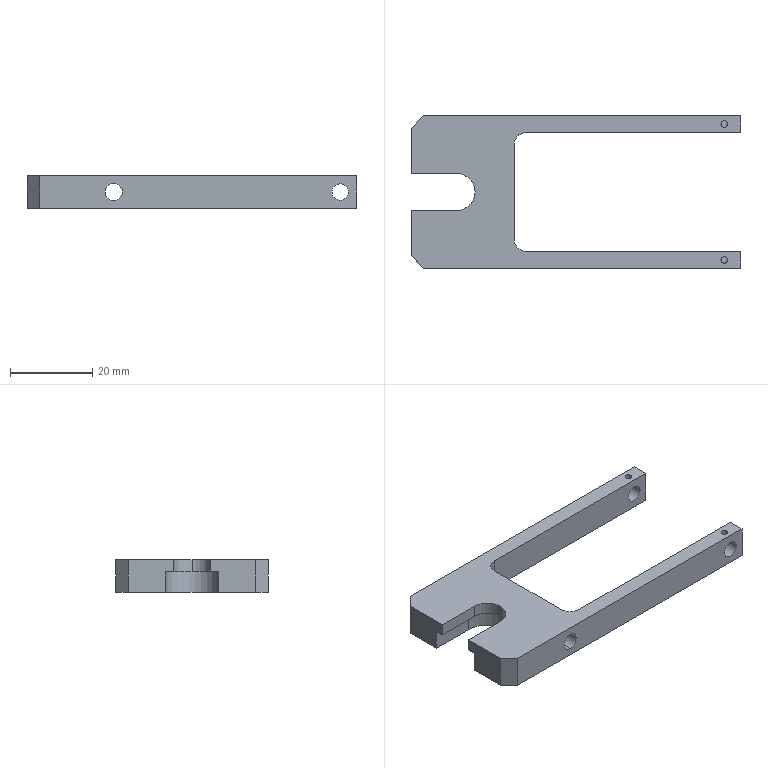Part | SolidWorks | features ICE 4, 3DProfileFeature 1, Chamfer 1, Extrusion 1, Fillet 1, HoleWzd 1, MirrorPattern 1 | 1 solid | 33 faces | box 80 x 37 x 8 mm | volume 8818 mm3 | plane 18 | cylinder 15 | commonest cylinder face diameters 1.6 x4 4 x4 4.2 x2 6 x2 9 x2 13 x1
STEP:
#1=CARTESIAN_POINT('',(50.2,16.5,1.833));
#2=VERTEX_POINT('',#1);
#3=CARTESIAN_POINT('',(51.8,16.5,1.833));
#4=VERTEX_POINT('',#3);
#5=CARTESIAN_POINT('',(50.2,16.5,1.833));
#6=CARTESIAN_POINT('',(50.2,16.395,1.833));
#7=CARTESIAN_POINT('',(50.221,16.289,1.843));
#8=CARTESIAN_POINT('',(50.302,16.095,1.875));
#9=CARTESIAN_POINT('',(50.361,16.008,1.897));
#10=CARTESIAN_POINT('',(50.508,15.861,1.94));
#11=CARTESIAN_POINT('',(50.595,15.802,1.961));
#12=CARTESIAN_POINT('',(50.789,15.721,1.991));
#13=CARTESIAN_POINT('',(50.894,15.7,2.));
#14=CARTESIAN_POINT('',(51.105,15.7,2.));
#15=CARTESIAN_POINT('',(51.211,15.721,1.991));
#16=CARTESIAN_POINT('',(51.404,15.802,1.961));
#17=CARTESIAN_POINT('',(51.492,15.861,1.94));
#18=CARTESIAN_POINT('',(51.712,16.081,1.875));
#19=CARTESIAN_POINT('',(51.8,16.286,1.833));
#20=CARTESIAN_POINT('',(51.8,16.5,1.833));
#21=B_SPLINE_CURVE_WITH_KNOTS('',3,(#5,#6,#7,#8,#9,#10,#11,#12,#13,#14,#15,#16,#17,#18,#19,#20),.UNSPECIFIED.,.F.,.F.,(4,2,2,2,2,2,2,4),(0.002528,0.002843,0.003159,0.003475,0.003791,0.004106,0.004422,0.005053),.UNSPECIFIED.);
#22=EDGE_CURVE('',#2,#4,#21,.T.);
#23=ORIENTED_EDGE('',*,*,#22,.F.);
#24=CARTESIAN_POINT('',(50.2,16.5,4.));
#25=VERTEX_POINT('',#24);
#26=CARTESIAN_POINT('',(50.2,16.5,4.));
#27=DIRECTION('',(0.,0.,1.));
#28=VECTOR('',#27,1000.);
#29=LINE('',#26,#28);
#30=EDGE_CURVE('',#2,#25,#29,.T.);
#31=ORIENTED_EDGE('',*,*,#30,.T.);
#32=CARTESIAN_POINT('',(51.8,16.5,4.));
#33=VERTEX_POINT('',#32);
#34=CARTESIAN_POINT('',(51.,16.5,4.));
#35=DIRECTION('',(0.,0.,1.));
#36=DIRECTION('',(1.,0.,0.));
#37=AXIS2_PLACEMENT_3D('',#34,#35,#36);
#38=CIRCLE('',#37,0.8);
#39=EDGE_CURVE('',#25,#33,#38,.T.);
#40=ORIENTED_EDGE('',*,*,#39,.T.);
#41=CARTESIAN_POINT('',(51.8,16.5,4.));
#42=DIRECTION('',(0.,0.,1.));
#43=VECTOR('',#42,1000.);
#44=LINE('',#41,#43);
#45=EDGE_CURVE('',#4,#33,#44,.T.);
#46=ORIENTED_EDGE('',*,*,#45,.F.);
#47=EDGE_LOOP('',(#23,#31,#40,#46));
#48=FACE_OUTER_BOUND('',#47,.T.);
#49=CARTESIAN_POINT('',(51.,16.5,4.));
#50=DIRECTION('',(0.,0.,1.));
#51=DIRECTION('',(1.,0.,0.));
#52=AXIS2_PLACEMENT_3D('',#49,#50,#51);
#53=CYLINDRICAL_SURFACE('',#52,0.8);
#54=ADVANCED_FACE('',(#48),#53,.F.);
#55=CARTESIAN_POINT('',(50.2,-16.5,1.833));
#56=VERTEX_POINT('',#55);
#57=CARTESIAN_POINT('',(51.8,-16.5,1.833));
#58=VERTEX_POINT('',#57);
#59=CARTESIAN_POINT('',(50.2,-16.5,1.833));
#60=CARTESIAN_POINT('',(50.2,-16.605,1.833));
#61=CARTESIAN_POINT('',(50.221,-16.711,1.843));
#62=CARTESIAN_POINT('',(50.302,-16.905,1.875));
#63=CARTESIAN_POINT('',(50.361,-16.992,1.897));
#64=CARTESIAN_POINT('',(50.508,-17.139,1.94));
#65=CARTESIAN_POINT('',(50.595,-17.198,1.961));
#66=CARTESIAN_POINT('',(50.789,-17.279,1.991));
#67=CARTESIAN_POINT('',(50.894,-17.3,2.));
#68=CARTESIAN_POINT('',(51.105,-17.3,2.));
#69=CARTESIAN_POINT('',(51.211,-17.279,1.991));
#70=CARTESIAN_POINT('',(51.404,-17.198,1.961));
#71=CARTESIAN_POINT('',(51.492,-17.139,1.94));
#72=CARTESIAN_POINT('',(51.712,-16.919,1.875));
#73=CARTESIAN_POINT('',(51.8,-16.714,1.833));
#74=CARTESIAN_POINT('',(51.8,-16.5,1.833));
#75=B_SPLINE_CURVE_WITH_KNOTS('',3,(#59,#60,#61,#62,#63,#64,#65,#66,#67,#68,#69,#70,#71,#72,#73,#74),.UNSPECIFIED.,.F.,.F.,(4,2,2,2,2,2,2,4),(0.002528,0.002843,0.003159,0.003475,0.003791,0.004106,0.004422,0.005053),.UNSPECIFIED.);
#76=EDGE_CURVE('',#56,#58,#75,.T.);
#77=ORIENTED_EDGE('',*,*,#76,.F.);
#78=CARTESIAN_POINT('',(50.2,-16.5,4.));
#79=VERTEX_POINT('',#78);
#80=CARTESIAN_POINT('',(50.2,-16.5,4.));
#81=DIRECTION('',(0.,0.,1.));
#82=VECTOR('',#81,1000.);
#83=LINE('',#80,#82);
#84=EDGE_CURVE('',#56,#79,#83,.T.);
#85=ORIENTED_EDGE('',*,*,#84,.T.);
#86=CARTESIAN_POINT('',(51.8,-16.5,4.));
#87=VERTEX_POINT('',#86);
#88=CARTESIAN_POINT('',(51.,-16.5,4.));
#89=DIRECTION('',(0.,0.,1.));
#90=DIRECTION('',(1.,0.,0.));
#91=AXIS2_PLACEMENT_3D('',#88,#89,#90);
#92=CIRCLE('',#91,0.8);
#93=EDGE_CURVE('',#79,#87,#92,.T.);
#94=ORIENTED_EDGE('',*,*,#93,.T.);
#95=CARTESIAN_POINT('',(51.8,-16.5,4.));
#96=DIRECTION('',(0.,0.,1.));
#97=VECTOR('',#96,1000.);
#98=LINE('',#95,#97);
#99=EDGE_CURVE('',#58,#87,#98,.T.);
#100=ORIENTED_EDGE('',*,*,#99,.F.);
#101=EDGE_LOOP('',(#77,#85,#94,#100));
#102=FACE_OUTER_BOUND('',#101,.T.);
#103=CARTESIAN_POINT('',(51.,-16.5,4.));
#104=DIRECTION('',(0.,0.,1.));
#105=DIRECTION('',(1.,0.,0.));
#106=AXIS2_PLACEMENT_3D('',#103,#104,#105);
#107=CYLINDRICAL_SURFACE('',#106,0.8);
#108=ADVANCED_FACE('',(#102),#107,.F.);
#109=CARTESIAN_POINT('',(-4.,18.5,-2.1));
#110=VERTEX_POINT('',#109);
#111=CARTESIAN_POINT('',(-4.,18.5,2.1));
#112=VERTEX_POINT('',#111);
#113=CARTESIAN_POINT('',(-4.,18.5,0.));
#114=DIRECTION('',(0.,1.,0.));
#115=DIRECTION('',(1.,0.,0.));
#116=AXIS2_PLACEMENT_3D('',#113,#114,#115);
#117=CIRCLE('',#116,2.1);
#118=EDGE_CURVE('',#110,#112,#117,.T.);
#119=ORIENTED_EDGE('',*,*,#118,.T.);
#120=CARTESIAN_POINT('',(-4.,-18.5,2.1));
#121=VERTEX_POINT('',#120);
#122=CARTESIAN_POINT('',(-4.,18.501,2.1));
#123=DIRECTION('',(0.,-1.,0.));
#124=VECTOR('',#123,1000.);
#125=LINE('',#122,#124);
#126=EDGE_CURVE('',#112,#121,#125,.T.);
#127=ORIENTED_EDGE('',*,*,#126,.T.);
#128=CARTESIAN_POINT('',(-4.,-18.5,-2.1));
#129=VERTEX_POINT('',#128);
#130=CARTESIAN_POINT('',(-4.,-18.5,0.));
#131=DIRECTION('',(0.,-1.,0.));
#132=DIRECTION('',(0.,0.,-1.));
#133=AXIS2_PLACEMENT_3D('',#130,#131,#132);
#134=CIRCLE('',#133,2.1);
#135=EDGE_CURVE('',#121,#129,#134,.T.);
#136=ORIENTED_EDGE('',*,*,#135,.T.);
#137=CARTESIAN_POINT('',(-4.,18.501,-2.1));
#138=DIRECTION('',(0.,-1.,0.));
#139=VECTOR('',#138,1000.);
#140=LINE('',#137,#139);
#141=EDGE_CURVE('',#110,#129,#140,.T.);
#142=ORIENTED_EDGE('',*,*,#141,.F.);
#143=EDGE_LOOP('',(#119,#127,#136,#142));
#144=FACE_OUTER_BOUND('',#143,.T.);
#145=CARTESIAN_POINT('',(-4.,18.501,0.));
#146=DIRECTION('',(0.,-1.,0.));
#147=DIRECTION('',(0.,0.,-1.));
#148=AXIS2_PLACEMENT_3D('',#145,#146,#147);
#149=CYLINDRICAL_SURFACE('',#148,2.1);
#150=ADVANCED_FACE('',(#144),#149,.F.);
#151=CARTESIAN_POINT('',(53.,14.5,0.));
#152=VERTEX_POINT('',#151);
#153=CARTESIAN_POINT('',(49.,14.5,0.));
#154=VERTEX_POINT('',#153);
#155=CARTESIAN_POINT('',(51.,14.5,0.));
#156=DIRECTION('',(0.,1.,0.));
#157=DIRECTION('',(0.,0.,1.));
#158=AXIS2_PLACEMENT_3D('',#155,#156,#157);
#159=CIRCLE('',#158,2.);
#160=EDGE_CURVE('',#152,#154,#159,.T.);
#161=ORIENTED_EDGE('',*,*,#160,.F.);
#162=CARTESIAN_POINT('',(53.,18.5,0.));
#163=VERTEX_POINT('',#162);
#164=CARTESIAN_POINT('',(53.,-24.157,0.));
#165=DIRECTION('',(0.,1.,0.));
#166=VECTOR('',#165,1000.);
#167=LINE('',#164,#166);
#168=EDGE_CURVE('',#152,#163,#167,.T.);
#169=ORIENTED_EDGE('',*,*,#168,.T.);
#170=CARTESIAN_POINT('',(49.,18.5,0.));
#171=VERTEX_POINT('',#170);
#172=CARTESIAN_POINT('',(51.,18.5,0.));
#173=DIRECTION('',(0.,1.,0.));
#174=DIRECTION('',(-1.,0.,0.));
#175=AXIS2_PLACEMENT_3D('',#172,#173,#174);
#176=CIRCLE('',#175,2.);
#177=EDGE_CURVE('',#163,#171,#176,.T.);
#178=ORIENTED_EDGE('',*,*,#177,.T.);
#179=CARTESIAN_POINT('',(49.,-24.157,0.));
#180=DIRECTION('',(0.,1.,0.));
#181=VECTOR('',#180,1000.);
#182=LINE('',#179,#181);
#183=EDGE_CURVE('',#154,#171,#182,.T.);
#184=ORIENTED_EDGE('',*,*,#183,.F.);
#185=EDGE_LOOP('',(#161,#169,#178,#184));
#186=FACE_OUTER_BOUND('',#185,.T.);
#187=CARTESIAN_POINT('',(51.,-24.157,0.));
#188=DIRECTION('',(0.,1.,0.));
#189=DIRECTION('',(-1.,0.,0.));
#190=AXIS2_PLACEMENT_3D('',#187,#188,#189);
#191=CYLINDRICAL_SURFACE('',#190,2.);
#192=ADVANCED_FACE('',(#186),#191,.F.);
#193=CARTESIAN_POINT('',(49.,-18.5,0.));
#194=VERTEX_POINT('',#193);
#195=CARTESIAN_POINT('',(53.,-18.5,0.));
#196=VERTEX_POINT('',#195);
#197=CARTESIAN_POINT('',(51.,-18.5,0.));
#198=DIRECTION('',(0.,-1.,0.));
#199=DIRECTION('',(0.,0.,1.));
#200=AXIS2_PLACEMENT_3D('',#197,#198,#199);
#201=CIRCLE('',#200,2.);
#202=EDGE_CURVE('',#194,#196,#201,.T.);
#203=ORIENTED_EDGE('',*,*,#202,.T.);
#204=CARTESIAN_POINT('',(53.,-14.5,0.));
#205=VERTEX_POINT('',#204);
#206=CARTESIAN_POINT('',(53.,-24.157,0.));
#207=DIRECTION('',(0.,1.,0.));
#208=VECTOR('',#207,1000.);
#209=LINE('',#206,#208);
#210=EDGE_CURVE('',#196,#205,#209,.T.);
#211=ORIENTED_EDGE('',*,*,#210,.T.);
#212=CARTESIAN_POINT('',(49.,-14.5,0.));
#213=VERTEX_POINT('',#212);
#214=CARTESIAN_POINT('',(51.,-14.5,0.));
#215=DIRECTION('',(0.,-1.,0.));
#216=DIRECTION('',(1.,0.,0.));
#217=AXIS2_PLACEMENT_3D('',#214,#215,#216);
#218=CIRCLE('',#217,2.);
#219=EDGE_CURVE('',#213,#205,#218,.T.);
#220=ORIENTED_EDGE('',*,*,#219,.F.);
#221=CARTESIAN_POINT('',(49.,-24.157,0.));
#222=DIRECTION('',(0.,1.,0.));
#223=VECTOR('',#222,1000.);
#224=LINE('',#221,#223);
#225=EDGE_CURVE('',#194,#213,#224,.T.);
#226=ORIENTED_EDGE('',*,*,#225,.F.);
#227=EDGE_LOOP('',(#203,#211,#220,#226));
#228=FACE_OUTER_BOUND('',#227,.T.);
#229=CARTESIAN_POINT('',(51.,-24.157,0.));
#230=DIRECTION('',(0.,1.,0.));
#231=DIRECTION('',(-1.,0.,0.));
#232=AXIS2_PLACEMENT_3D('',#229,#230,#231);
#233=CYLINDRICAL_SURFACE('',#232,2.);
#234=ADVANCED_FACE('',(#228),#233,.F.);
#235=CARTESIAN_POINT('',(-9.5,0.,1.));
#236=VERTEX_POINT('',#235);
#237=CARTESIAN_POINT('',(-14.,4.5,1.));
#238=VERTEX_POINT('',#237);
#239=CARTESIAN_POINT('',(-14.,0.,1.));
#240=DIRECTION('',(0.,0.,1.));
#241=DIRECTION('',(-1.,0.,0.));
#242=AXIS2_PLACEMENT_3D('',#239,#240,#241);
#243=CIRCLE('',#242,4.5);
#244=EDGE_CURVE('',#236,#238,#243,.T.);
#245=ORIENTED_EDGE('',*,*,#244,.F.);
#246=CARTESIAN_POINT('',(-9.5,0.,4.));
#247=VERTEX_POINT('',#246);
#248=CARTESIAN_POINT('',(-9.5,0.,-4.001));
#249=DIRECTION('',(0.,0.,1.));
#250=VECTOR('',#249,1000.);
#251=LINE('',#248,#250);
#252=EDGE_CURVE('',#236,#247,#251,.T.);
#253=ORIENTED_EDGE('',*,*,#252,.T.);
#254=CARTESIAN_POINT('',(-14.,4.5,4.));
#255=VERTEX_POINT('',#254);
#256=CARTESIAN_POINT('',(-14.,0.,4.));
#257=DIRECTION('',(0.,0.,1.));
#258=DIRECTION('',(-1.,0.,0.));
#259=AXIS2_PLACEMENT_3D('',#256,#257,#258);
#260=CIRCLE('',#259,4.5);
#261=EDGE_CURVE('',#247,#255,#260,.T.);
#262=ORIENTED_EDGE('',*,*,#261,.T.);
#263=CARTESIAN_POINT('',(-14.,4.5,-4.001));
#264=DIRECTION('',(0.,0.,1.));
#265=VECTOR('',#264,1000.);
#266=LINE('',#263,#265);
#267=EDGE_CURVE('',#238,#255,#266,.T.);
#268=ORIENTED_EDGE('',*,*,#267,.F.);
#269=EDGE_LOOP('',(#245,#253,#262,#268));
#270=FACE_OUTER_BOUND('',#269,.T.);
#271=CARTESIAN_POINT('',(-14.,0.,-4.001));
#272=DIRECTION('',(0.,0.,1.));
#273=DIRECTION('',(1.,0.,0.));
#274=AXIS2_PLACEMENT_3D('',#271,#272,#273);
#275=CYLINDRICAL_SURFACE('',#274,4.5);
#276=ADVANCED_FACE('',(#270),#275,.F.);
#277=CARTESIAN_POINT('',(-25.,4.5,1.));
#278=VERTEX_POINT('',#277);
#279=CARTESIAN_POINT('',(-25.,4.5,1.));
#280=DIRECTION('',(-1.,0.,0.));
#281=VECTOR('',#280,1000.);
#282=LINE('',#279,#281);
#283=EDGE_CURVE('',#238,#278,#282,.T.);
#284=ORIENTED_EDGE('',*,*,#283,.F.);
#285=ORIENTED_EDGE('',*,*,#267,.T.);
#286=CARTESIAN_POINT('',(-25.,4.5,4.));
#287=VERTEX_POINT('',#286);
#288=CARTESIAN_POINT('',(-25.,4.5,4.));
#289=DIRECTION('',(-1.,0.,0.));
#290=VECTOR('',#289,1000.);
#291=LINE('',#288,#290);
#292=EDGE_CURVE('',#255,#287,#291,.T.);
#293=ORIENTED_EDGE('',*,*,#292,.T.);
#294=CARTESIAN_POINT('',(-25.,4.5,-4.001));
#295=DIRECTION('',(0.,0.,1.));
#296=VECTOR('',#295,1000.);
#297=LINE('',#294,#296);
#298=EDGE_CURVE('',#278,#287,#297,.T.);
#299=ORIENTED_EDGE('',*,*,#298,.F.);
#300=EDGE_LOOP('',(#284,#285,#293,#299));
#301=FACE_OUTER_BOUND('',#300,.T.);
#302=CARTESIAN_POINT('',(-25.,4.5,-4.001));
#303=DIRECTION('',(0.,1.,0.));
#304=DIRECTION('',(-1.,0.,0.));
#305=AXIS2_PLACEMENT_3D('',#302,#303,#304);
#306=PLANE('',#305);
#307=ADVANCED_FACE('',(#301),#306,.F.);
#308=ORIENTED_EDGE('',*,*,#252,.F.);
#309=CARTESIAN_POINT('',(-14.,-4.5,1.));
#310=VERTEX_POINT('',#309);
#311=CARTESIAN_POINT('',(-14.,0.,1.));
#312=DIRECTION('',(0.,0.,1.));
#313=DIRECTION('',(-1.,0.,0.));
#314=AXIS2_PLACEMENT_3D('',#311,#312,#313);
#315=CIRCLE('',#314,4.5);
#316=EDGE_CURVE('',#310,#236,#315,.T.);
#317=ORIENTED_EDGE('',*,*,#316,.F.);
#318=CARTESIAN_POINT('',(-14.,-4.5,4.));
#319=VERTEX_POINT('',#318);
#320=CARTESIAN_POINT('',(-14.,-4.5,-4.001));
#321=DIRECTION('',(0.,0.,1.));
#322=VECTOR('',#321,1000.);
#323=LINE('',#320,#322);
#324=EDGE_CURVE('',#310,#319,#323,.T.);
#325=ORIENTED_EDGE('',*,*,#324,.T.);
#326=CARTESIAN_POINT('',(-14.,0.,4.));
#327=DIRECTION('',(0.,0.,1.));
#328=DIRECTION('',(-1.,0.,0.));
#329=AXIS2_PLACEMENT_3D('',#326,#327,#328);
#330=CIRCLE('',#329,4.5);
#331=EDGE_CURVE('',#319,#247,#330,.T.);
#332=ORIENTED_EDGE('',*,*,#331,.T.);
#333=EDGE_LOOP('',(#308,#317,#325,#332));
#334=FACE_OUTER_BOUND('',#333,.T.);
#335=CARTESIAN_POINT('',(-14.,0.,-4.001));
#336=DIRECTION('',(0.,0.,1.));
#337=DIRECTION('',(1.,0.,0.));
#338=AXIS2_PLACEMENT_3D('',#335,#336,#337);
#339=CYLINDRICAL_SURFACE('',#338,4.5);
#340=ADVANCED_FACE('',(#334),#339,.F.);
#341=CARTESIAN_POINT('',(-25.,-4.5,1.));
#342=VERTEX_POINT('',#341);
#343=CARTESIAN_POINT('',(-14.,-4.5,1.));
#344=DIRECTION('',(1.,0.,0.));
#345=VECTOR('',#344,1000.);
#346=LINE('',#343,#345);
#347=EDGE_CURVE('',#342,#310,#346,.T.);
#348=ORIENTED_EDGE('',*,*,#347,.F.);
#349=CARTESIAN_POINT('',(-25.,-4.5,4.));
#350=VERTEX_POINT('',#349);
#351=CARTESIAN_POINT('',(-25.,-4.5,-4.001));
#352=DIRECTION('',(0.,0.,1.));
#353=VECTOR('',#352,1000.);
#354=LINE('',#351,#353);
#355=EDGE_CURVE('',#342,#350,#354,.T.);
#356=ORIENTED_EDGE('',*,*,#355,.T.);
#357=CARTESIAN_POINT('',(-14.,-4.5,4.));
#358=DIRECTION('',(1.,0.,0.));
#359=VECTOR('',#358,1000.);
#360=LINE('',#357,#359);
#361=EDGE_CURVE('',#350,#319,#360,.T.);
#362=ORIENTED_EDGE('',*,*,#361,.T.);
#363=ORIENTED_EDGE('',*,*,#324,.F.);
#364=EDGE_LOOP('',(#348,#356,#362,#363));
#365=FACE_OUTER_BOUND('',#364,.T.);
#366=CARTESIAN_POINT('',(-14.,-4.5,-4.001));
#367=DIRECTION('',(0.,-1.,0.));
#368=DIRECTION('',(1.,0.,0.));
#369=AXIS2_PLACEMENT_3D('',#366,#367,#368);
#370=PLANE('',#369);
#371=ADVANCED_FACE('',(#365),#370,.F.);
#372=CARTESIAN_POINT('',(-25.,15.5,4.));
#373=VERTEX_POINT('',#372);
#374=CARTESIAN_POINT('',(-25.,18.5,4.));
#375=DIRECTION('',(0.,-1.,0.));
#376=VECTOR('',#375,1000.);
#377=LINE('',#374,#376);
#378=EDGE_CURVE('',#373,#287,#377,.T.);
#379=ORIENTED_EDGE('',*,*,#378,.F.);
#380=CARTESIAN_POINT('',(-25.,15.5,-4.));
#381=VERTEX_POINT('',#380);
#382=CARTESIAN_POINT('',(-25.,15.5,4.));
#383=DIRECTION('',(0.,0.,-1.));
#384=VECTOR('',#383,1000.);
#385=LINE('',#382,#384);
#386=EDGE_CURVE('',#373,#381,#385,.T.);
#387=ORIENTED_EDGE('',*,*,#386,.T.);
#388=CARTESIAN_POINT('',(-25.,6.5,-4.));
#389=VERTEX_POINT('',#388);
#390=CARTESIAN_POINT('',(-25.,18.5,-4.));
#391=DIRECTION('',(0.,-1.,0.));
#392=VECTOR('',#391,1000.);
#393=LINE('',#390,#392);
#394=EDGE_CURVE('',#381,#389,#393,.T.);
#395=ORIENTED_EDGE('',*,*,#394,.T.);
#396=CARTESIAN_POINT('',(-25.,6.5,1.));
#397=VERTEX_POINT('',#396);
#398=CARTESIAN_POINT('',(-25.,6.5,1.));
#399=DIRECTION('',(0.,0.,-1.));
#400=VECTOR('',#399,1000.);
#401=LINE('',#398,#400);
#402=EDGE_CURVE('',#397,#389,#401,.T.);
#403=ORIENTED_EDGE('',*,*,#402,.F.);
#404=CARTESIAN_POINT('',(-25.,-6.5,1.));
#405=DIRECTION('',(0.,1.,0.));
#406=VECTOR('',#405,1000.);
#407=LINE('',#404,#406);
#408=EDGE_CURVE('',#278,#397,#407,.T.);
#409=ORIENTED_EDGE('',*,*,#408,.F.);
#410=ORIENTED_EDGE('',*,*,#298,.T.);
#411=EDGE_LOOP('',(#379,#387,#395,#403,#409,#410));
#412=FACE_OUTER_BOUND('',#411,.T.);
#413=CARTESIAN_POINT('',(-25.,18.5,4.));
#414=DIRECTION('',(1.,0.,0.));
#415=DIRECTION('',(0.,1.,0.));
#416=AXIS2_PLACEMENT_3D('',#413,#414,#415);
#417=PLANE('',#416);
#418=ADVANCED_FACE('',(#412),#417,.F.);
#419=CARTESIAN_POINT('',(51.,-16.5,4.));
#420=DIRECTION('',(0.,0.,1.));
#421=DIRECTION('',(1.,0.,0.));
#422=AXIS2_PLACEMENT_3D('',#419,#420,#421);
#423=CIRCLE('',#422,0.8);
#424=EDGE_CURVE('',#87,#79,#423,.T.);
#425=ORIENTED_EDGE('',*,*,#424,.F.);
#426=ORIENTED_EDGE('',*,*,#93,.F.);
#427=EDGE_LOOP('',(#425,#426));
#428=FACE_BOUND('',#427,.T.);
#429=CARTESIAN_POINT('',(55.,18.5,4.));
#430=VERTEX_POINT('',#429);
#431=CARTESIAN_POINT('',(-22.,18.5,4.));
#432=VERTEX_POINT('',#431);
#433=CARTESIAN_POINT('',(55.,18.5,4.));
#434=DIRECTION('',(-1.,0.,0.));
#435=VECTOR('',#434,1000.);
#436=LINE('',#433,#435);
#437=EDGE_CURVE('',#430,#432,#436,.T.);
#438=ORIENTED_EDGE('',*,*,#437,.T.);
#439=CARTESIAN_POINT('',(-25.,15.5,4.));
#440=DIRECTION('',(-0.7071,-0.7071,0.));
#441=VECTOR('',#440,1000.);
#442=LINE('',#439,#441);
#443=EDGE_CURVE('',#432,#373,#442,.T.);
#444=ORIENTED_EDGE('',*,*,#443,.T.);
#445=ORIENTED_EDGE('',*,*,#378,.T.);
#446=ORIENTED_EDGE('',*,*,#292,.F.);
#447=ORIENTED_EDGE('',*,*,#261,.F.);
#448=ORIENTED_EDGE('',*,*,#331,.F.);
#449=ORIENTED_EDGE('',*,*,#361,.F.);
#450=CARTESIAN_POINT('',(-25.,-15.5,4.));
#451=VERTEX_POINT('',#450);
#452=CARTESIAN_POINT('',(-25.,18.5,4.));
#453=DIRECTION('',(0.,-1.,0.));
#454=VECTOR('',#453,1000.);
#455=LINE('',#452,#454);
#456=EDGE_CURVE('',#350,#451,#455,.T.);
#457=ORIENTED_EDGE('',*,*,#456,.T.);
#458=CARTESIAN_POINT('',(-22.,-18.5,4.));
#459=VERTEX_POINT('',#458);
#460=CARTESIAN_POINT('',(-22.,-18.5,4.));
#461=DIRECTION('',(0.7071,-0.7071,0.));
#462=VECTOR('',#461,1000.);
#463=LINE('',#460,#462);
#464=EDGE_CURVE('',#451,#459,#463,.T.);
#465=ORIENTED_EDGE('',*,*,#464,.T.);
#466=CARTESIAN_POINT('',(55.,-18.5,4.));
#467=VERTEX_POINT('',#466);
#468=CARTESIAN_POINT('',(-25.,-18.5,4.));
#469=DIRECTION('',(1.,0.,0.));
#470=VECTOR('',#469,1000.);
#471=LINE('',#468,#470);
#472=EDGE_CURVE('',#459,#467,#471,.T.);
#473=ORIENTED_EDGE('',*,*,#472,.T.);
#474=CARTESIAN_POINT('',(55.,-14.5,4.));
#475=VERTEX_POINT('',#474);
#476=CARTESIAN_POINT('',(55.,-18.5,4.));
#477=DIRECTION('',(0.,1.,0.));
#478=VECTOR('',#477,1000.);
#479=LINE('',#476,#478);
#480=EDGE_CURVE('',#467,#475,#479,.T.);
#481=ORIENTED_EDGE('',*,*,#480,.T.);
#482=CARTESIAN_POINT('',(3.,-14.5,4.));
#483=VERTEX_POINT('',#482);
#484=CARTESIAN_POINT('',(55.,-14.5,4.));
#485=DIRECTION('',(-1.,0.,0.));
#486=VECTOR('',#485,1000.);
#487=LINE('',#484,#486);
#488=EDGE_CURVE('',#475,#483,#487,.T.);
#489=ORIENTED_EDGE('',*,*,#488,.T.);
#490=CARTESIAN_POINT('',(0.,-11.5,4.));
#491=VERTEX_POINT('',#490);
#492=CARTESIAN_POINT('',(3.,-11.5,4.));
#493=DIRECTION('',(0.,0.,-1.));
#494=DIRECTION('',(-1.,0.,0.));
#495=AXIS2_PLACEMENT_3D('',#492,#493,#494);
#496=CIRCLE('',#495,3.);
#497=EDGE_CURVE('',#483,#491,#496,.T.);
#498=ORIENTED_EDGE('',*,*,#497,.T.);
#499=CARTESIAN_POINT('',(0.,11.5,4.));
#500=VERTEX_POINT('',#499);
#501=CARTESIAN_POINT('',(0.,-14.5,4.));
#502=DIRECTION('',(0.,1.,0.));
#503=VECTOR('',#502,1000.);
#504=LINE('',#501,#503);
#505=EDGE_CURVE('',#491,#500,#504,.T.);
#506=ORIENTED_EDGE('',*,*,#505,.T.);
#507=CARTESIAN_POINT('',(3.,14.5,4.));
#508=VERTEX_POINT('',#507);
#509=CARTESIAN_POINT('',(3.,11.5,4.));
#510=DIRECTION('',(0.,0.,-1.));
#511=DIRECTION('',(-1.,0.,0.));
#512=AXIS2_PLACEMENT_3D('',#509,#510,#511);
#513=CIRCLE('',#512,3.);
#514=EDGE_CURVE('',#500,#508,#513,.T.);
#515=ORIENTED_EDGE('',*,*,#514,.T.);
#516=CARTESIAN_POINT('',(55.,14.5,4.));
#517=VERTEX_POINT('',#516);
#518=CARTESIAN_POINT('',(0.,14.5,4.));
#519=DIRECTION('',(1.,0.,0.));
#520=VECTOR('',#519,1000.);
#521=LINE('',#518,#520);
#522=EDGE_CURVE('',#508,#517,#521,.T.);
#523=ORIENTED_EDGE('',*,*,#522,.T.);
#524=CARTESIAN_POINT('',(55.,14.5,4.));
#525=DIRECTION('',(0.,1.,0.));
#526=VECTOR('',#525,1000.);
#527=LINE('',#524,#526);
#528=EDGE_CURVE('',#517,#430,#527,.T.);
#529=ORIENTED_EDGE('',*,*,#528,.T.);
#530=EDGE_LOOP('',(#438,#444,#445,#446,#447,#448,#449,#457,#465,#473,#481,#489,#498,#506,#515,#523,#529));
#531=FACE_OUTER_BOUND('',#530,.T.);
#532=CARTESIAN_POINT('',(51.,16.5,4.));
#533=DIRECTION('',(0.,0.,1.));
#534=DIRECTION('',(1.,0.,0.));
#535=AXIS2_PLACEMENT_3D('',#532,#533,#534);
#536=CIRCLE('',#535,0.8);
#537=EDGE_CURVE('',#33,#25,#536,.T.);
#538=ORIENTED_EDGE('',*,*,#537,.F.);
#539=ORIENTED_EDGE('',*,*,#39,.F.);
#540=EDGE_LOOP('',(#538,#539));
#541=FACE_BOUND('',#540,.T.);
#542=CARTESIAN_POINT('',(0.,0.,4.));
#543=DIRECTION('',(0.,0.,-1.));
#544=DIRECTION('',(-1.,0.,0.));
#545=AXIS2_PLACEMENT_3D('',#542,#543,#544);
#546=PLANE('',#545);
#547=ADVANCED_FACE('',(#428,#531,#541),#546,.F.);
#548=ORIENTED_EDGE('',*,*,#505,.F.);
#549=CARTESIAN_POINT('',(0.,-11.5,-4.));
#550=VERTEX_POINT('',#549);
#551=CARTESIAN_POINT('',(0.,-11.5,-4.));
#552=DIRECTION('',(0.,0.,-1.));
#553=VECTOR('',#552,1000.);
#554=LINE('',#551,#553);
#555=EDGE_CURVE('',#491,#550,#554,.T.);
#556=ORIENTED_EDGE('',*,*,#555,.T.);
#557=CARTESIAN_POINT('',(0.,11.5,-4.));
#558=VERTEX_POINT('',#557);
#559=CARTESIAN_POINT('',(0.,0.,-4.));
#560=DIRECTION('',(0.,1.,0.));
#561=VECTOR('',#560,1000.);
#562=LINE('',#559,#561);
#563=EDGE_CURVE('',#550,#558,#562,.T.);
#564=ORIENTED_EDGE('',*,*,#563,.T.);
#565=CARTESIAN_POINT('',(0.,11.5,4.));
#566=DIRECTION('',(0.,0.,1.));
#567=VECTOR('',#566,1000.);
#568=LINE('',#565,#567);
#569=EDGE_CURVE('',#558,#500,#568,.T.);
#570=ORIENTED_EDGE('',*,*,#569,.T.);
#571=EDGE_LOOP('',(#548,#556,#564,#570));
#572=FACE_OUTER_BOUND('',#571,.T.);
#573=CARTESIAN_POINT('',(0.,0.,4.));
#574=DIRECTION('',(-1.,0.,0.));
#575=DIRECTION('',(0.,0.,1.));
#576=AXIS2_PLACEMENT_3D('',#573,#574,#575);
#577=PLANE('',#576);
#578=ADVANCED_FACE('',(#572),#577,.F.);
#579=CARTESIAN_POINT('',(51.,14.5,0.));
#580=DIRECTION('',(0.,1.,0.));
#581=DIRECTION('',(0.,0.,1.));
#582=AXIS2_PLACEMENT_3D('',#579,#580,#581);
#583=CIRCLE('',#582,2.);
#584=EDGE_CURVE('',#154,#152,#583,.T.);
#585=ORIENTED_EDGE('',*,*,#584,.T.);
#586=ORIENTED_EDGE('',*,*,#160,.T.);
#587=EDGE_LOOP('',(#585,#586));
#588=FACE_BOUND('',#587,.T.);
#589=ORIENTED_EDGE('',*,*,#522,.F.);
#590=CARTESIAN_POINT('',(3.,14.5,-4.));
#591=VERTEX_POINT('',#590);
#592=CARTESIAN_POINT('',(3.,14.5,-4.));
#593=DIRECTION('',(0.,0.,-1.));
#594=VECTOR('',#593,1000.);
#595=LINE('',#592,#594);
#596=EDGE_CURVE('',#508,#591,#595,.T.);
#597=ORIENTED_EDGE('',*,*,#596,.T.);
#598=CARTESIAN_POINT('',(55.,14.5,-4.));
#599=VERTEX_POINT('',#598);
#600=CARTESIAN_POINT('',(0.,14.5,-4.));
#601=DIRECTION('',(1.,0.,0.));
#602=VECTOR('',#601,1000.);
#603=LINE('',#600,#602);
#604=EDGE_CURVE('',#591,#599,#603,.T.);
#605=ORIENTED_EDGE('',*,*,#604,.T.);
#606=CARTESIAN_POINT('',(55.,14.5,4.));
#607=DIRECTION('',(0.,0.,-1.));
#608=VECTOR('',#607,1000.);
#609=LINE('',#606,#608);
#610=EDGE_CURVE('',#517,#599,#609,.T.);
#611=ORIENTED_EDGE('',*,*,#610,.F.);
#612=EDGE_LOOP('',(#589,#597,#605,#611));
#613=FACE_OUTER_BOUND('',#612,.T.);
#614=CARTESIAN_POINT('',(0.,14.5,4.));
#615=DIRECTION('',(0.,1.,0.));
#616=DIRECTION('',(0.,0.,1.));
#617=AXIS2_PLACEMENT_3D('',#614,#615,#616);
#618=PLANE('',#617);
#619=ADVANCED_FACE('',(#588,#613),#618,.F.);
#620=CARTESIAN_POINT('',(55.,18.5,-4.));
#621=VERTEX_POINT('',#620);
#622=CARTESIAN_POINT('',(55.,14.5,-4.));
#623=DIRECTION('',(0.,1.,0.));
#624=VECTOR('',#623,1000.);
#625=LINE('',#622,#624);
#626=EDGE_CURVE('',#599,#621,#625,.T.);
#627=ORIENTED_EDGE('',*,*,#626,.T.);
#628=CARTESIAN_POINT('',(55.,18.5,4.));
#629=DIRECTION('',(0.,0.,-1.));
#630=VECTOR('',#629,1000.);
#631=LINE('',#628,#630);
#632=EDGE_CURVE('',#430,#621,#631,.T.);
#633=ORIENTED_EDGE('',*,*,#632,.F.);
#634=ORIENTED_EDGE('',*,*,#528,.F.);
#635=ORIENTED_EDGE('',*,*,#610,.T.);
#636=EDGE_LOOP('',(#627,#633,#634,#635));
#637=FACE_OUTER_BOUND('',#636,.T.);
#638=CARTESIAN_POINT('',(55.,14.5,4.));
#639=DIRECTION('',(-1.,0.,0.));
#640=DIRECTION('',(0.,0.,1.));
#641=AXIS2_PLACEMENT_3D('',#638,#639,#640);
#642=PLANE('',#641);
#643=ADVANCED_FACE('',(#637),#642,.F.);
#644=ORIENTED_EDGE('',*,*,#118,.F.);
#645=CARTESIAN_POINT('',(-4.,18.5,0.));
#646=DIRECTION('',(0.,1.,0.));
#647=DIRECTION('',(1.,0.,0.));
#648=AXIS2_PLACEMENT_3D('',#645,#646,#647);
#649=CIRCLE('',#648,2.1);
#650=EDGE_CURVE('',#112,#110,#649,.T.);
#651=ORIENTED_EDGE('',*,*,#650,.F.);
#652=EDGE_LOOP('',(#644,#651));
#653=FACE_BOUND('',#652,.T.);
#654=CARTESIAN_POINT('',(51.,18.5,0.));
#655=DIRECTION('',(0.,1.,0.));
#656=DIRECTION('',(-1.,0.,0.));
#657=AXIS2_PLACEMENT_3D('',#654,#655,#656);
#658=CIRCLE('',#657,2.);
#659=EDGE_CURVE('',#171,#163,#658,.T.);
#660=ORIENTED_EDGE('',*,*,#659,.F.);
#661=ORIENTED_EDGE('',*,*,#177,.F.);
#662=EDGE_LOOP('',(#660,#661));
#663=FACE_BOUND('',#662,.T.);
#664=CARTESIAN_POINT('',(-22.,18.5,-4.));
#665=VERTEX_POINT('',#664);
#666=CARTESIAN_POINT('',(55.,18.5,-4.));
#667=DIRECTION('',(-1.,0.,0.));
#668=VECTOR('',#667,1000.);
#669=LINE('',#666,#668);
#670=EDGE_CURVE('',#621,#665,#669,.T.);
#671=ORIENTED_EDGE('',*,*,#670,.T.);
#672=CARTESIAN_POINT('',(-22.,18.5,4.));
#673=DIRECTION('',(0.,0.,1.));
#674=VECTOR('',#673,1000.);
#675=LINE('',#672,#674);
#676=EDGE_CURVE('',#665,#432,#675,.T.);
#677=ORIENTED_EDGE('',*,*,#676,.T.);
#678=ORIENTED_EDGE('',*,*,#437,.F.);
#679=ORIENTED_EDGE('',*,*,#632,.T.);
#680=EDGE_LOOP('',(#671,#677,#678,#679));
#681=FACE_OUTER_BOUND('',#680,.T.);
#682=CARTESIAN_POINT('',(55.,18.5,4.));
#683=DIRECTION('',(0.,-1.,0.));
#684=DIRECTION('',(1.,0.,0.));
#685=AXIS2_PLACEMENT_3D('',#682,#683,#684);
#686=PLANE('',#685);
#687=ADVANCED_FACE('',(#653,#663,#681),#686,.F.);
#688=CARTESIAN_POINT('',(-25.,-6.5,-4.));
#689=VERTEX_POINT('',#688);
#690=CARTESIAN_POINT('',(-25.,-15.5,-4.));
#691=VERTEX_POINT('',#690);
#692=CARTESIAN_POINT('',(-25.,18.5,-4.));
#693=DIRECTION('',(0.,-1.,0.));
#694=VECTOR('',#693,1000.);
#695=LINE('',#692,#694);
#696=EDGE_CURVE('',#689,#691,#695,.T.);
#697=ORIENTED_EDGE('',*,*,#696,.T.);
#698=CARTESIAN_POINT('',(-25.,-15.5,4.));
#699=DIRECTION('',(0.,0.,1.));
#700=VECTOR('',#699,1000.);
#701=LINE('',#698,#700);
#702=EDGE_CURVE('',#691,#451,#701,.T.);
#703=ORIENTED_EDGE('',*,*,#702,.T.);
#704=ORIENTED_EDGE('',*,*,#456,.F.);
#705=ORIENTED_EDGE('',*,*,#355,.F.);
#706=CARTESIAN_POINT('',(-25.,-6.5,1.));
#707=VERTEX_POINT('',#706);
#708=CARTESIAN_POINT('',(-25.,-6.5,1.));
#709=DIRECTION('',(0.,1.,0.));
#710=VECTOR('',#709,1000.);
#711=LINE('',#708,#710);
#712=EDGE_CURVE('',#707,#342,#711,.T.);
#713=ORIENTED_EDGE('',*,*,#712,.F.);
#714=CARTESIAN_POINT('',(-25.,-6.5,1.));
#715=DIRECTION('',(0.,0.,-1.));
#716=VECTOR('',#715,1000.);
#717=LINE('',#714,#716);
#718=EDGE_CURVE('',#707,#689,#717,.T.);
#719=ORIENTED_EDGE('',*,*,#718,.T.);
#720=EDGE_LOOP('',(#697,#703,#704,#705,#713,#719));
#721=FACE_OUTER_BOUND('',#720,.T.);
#722=CARTESIAN_POINT('',(-25.,18.5,4.));
#723=DIRECTION('',(1.,0.,0.));
#724=DIRECTION('',(0.,1.,0.));
#725=AXIS2_PLACEMENT_3D('',#722,#723,#724);
#726=PLANE('',#725);
#727=ADVANCED_FACE('',(#721),#726,.F.);
#728=CARTESIAN_POINT('',(-4.,-18.5,0.));
#729=DIRECTION('',(0.,-1.,0.));
#730=DIRECTION('',(0.,0.,-1.));
#731=AXIS2_PLACEMENT_3D('',#728,#729,#730);
#732=CIRCLE('',#731,2.1);
#733=EDGE_CURVE('',#129,#121,#732,.T.);
#734=ORIENTED_EDGE('',*,*,#733,.F.);
#735=ORIENTED_EDGE('',*,*,#135,.F.);
#736=EDGE_LOOP('',(#734,#735));
#737=FACE_BOUND('',#736,.T.);
#738=ORIENTED_EDGE('',*,*,#202,.F.);
#739=CARTESIAN_POINT('',(51.,-18.5,0.));
#740=DIRECTION('',(0.,-1.,0.));
#741=DIRECTION('',(0.,0.,1.));
#742=AXIS2_PLACEMENT_3D('',#739,#740,#741);
#743=CIRCLE('',#742,2.);
#744=EDGE_CURVE('',#196,#194,#743,.T.);
#745=ORIENTED_EDGE('',*,*,#744,.F.);
#746=EDGE_LOOP('',(#738,#745));
#747=FACE_BOUND('',#746,.T.);
#748=ORIENTED_EDGE('',*,*,#472,.F.);
#749=CARTESIAN_POINT('',(-22.,-18.5,-4.));
#750=VERTEX_POINT('',#749);
#751=CARTESIAN_POINT('',(-22.,-18.5,4.));
#752=DIRECTION('',(0.,0.,-1.));
#753=VECTOR('',#752,1000.);
#754=LINE('',#751,#753);
#755=EDGE_CURVE('',#459,#750,#754,.T.);
#756=ORIENTED_EDGE('',*,*,#755,.T.);
#757=CARTESIAN_POINT('',(55.,-18.5,-4.));
#758=VERTEX_POINT('',#757);
#759=CARTESIAN_POINT('',(-25.,-18.5,-4.));
#760=DIRECTION('',(1.,0.,0.));
#761=VECTOR('',#760,1000.);
#762=LINE('',#759,#761);
#763=EDGE_CURVE('',#750,#758,#762,.T.);
#764=ORIENTED_EDGE('',*,*,#763,.T.);
#765=CARTESIAN_POINT('',(55.,-18.5,4.));
#766=DIRECTION('',(0.,0.,-1.));
#767=VECTOR('',#766,1000.);
#768=LINE('',#765,#767);
#769=EDGE_CURVE('',#467,#758,#768,.T.);
#770=ORIENTED_EDGE('',*,*,#769,.F.);
#771=EDGE_LOOP('',(#748,#756,#764,#770));
#772=FACE_OUTER_BOUND('',#771,.T.);
#773=CARTESIAN_POINT('',(-25.,-18.5,4.));
#774=DIRECTION('',(0.,1.,0.));
#775=DIRECTION('',(0.,0.,1.));
#776=AXIS2_PLACEMENT_3D('',#773,#774,#775);
#777=PLANE('',#776);
#778=ADVANCED_FACE('',(#737,#747,#772),#777,.F.);
#779=CARTESIAN_POINT('',(55.,-14.5,-4.));
#780=VERTEX_POINT('',#779);
#781=CARTESIAN_POINT('',(55.,-18.5,-4.));
#782=DIRECTION('',(0.,1.,0.));
#783=VECTOR('',#782,1000.);
#784=LINE('',#781,#783);
#785=EDGE_CURVE('',#758,#780,#784,.T.);
#786=ORIENTED_EDGE('',*,*,#785,.T.);
#787=CARTESIAN_POINT('',(55.,-14.5,4.));
#788=DIRECTION('',(0.,0.,-1.));
#789=VECTOR('',#788,1000.);
#790=LINE('',#787,#789);
#791=EDGE_CURVE('',#475,#780,#790,.T.);
#792=ORIENTED_EDGE('',*,*,#791,.F.);
#793=ORIENTED_EDGE('',*,*,#480,.F.);
#794=ORIENTED_EDGE('',*,*,#769,.T.);
#795=EDGE_LOOP('',(#786,#792,#793,#794));
#796=FACE_OUTER_BOUND('',#795,.T.);
#797=CARTESIAN_POINT('',(55.,-18.5,4.));
#798=DIRECTION('',(-1.,0.,0.));
#799=DIRECTION('',(0.,0.,1.));
#800=AXIS2_PLACEMENT_3D('',#797,#798,#799);
#801=PLANE('',#800);
#802=ADVANCED_FACE('',(#796),#801,.F.);
#803=ORIENTED_EDGE('',*,*,#219,.T.);
#804=CARTESIAN_POINT('',(51.,-14.5,0.));
#805=DIRECTION('',(0.,-1.,0.));
#806=DIRECTION('',(1.,0.,0.));
#807=AXIS2_PLACEMENT_3D('',#804,#805,#806);
#808=CIRCLE('',#807,2.);
#809=EDGE_CURVE('',#205,#213,#808,.T.);
#810=ORIENTED_EDGE('',*,*,#809,.T.);
#811=EDGE_LOOP('',(#803,#810));
#812=FACE_BOUND('',#811,.T.);
#813=CARTESIAN_POINT('',(3.,-14.5,-4.));
#814=VERTEX_POINT('',#813);
#815=CARTESIAN_POINT('',(55.,-14.5,-4.));
#816=DIRECTION('',(-1.,0.,0.));
#817=VECTOR('',#816,1000.);
#818=LINE('',#815,#817);
#819=EDGE_CURVE('',#780,#814,#818,.T.);
#820=ORIENTED_EDGE('',*,*,#819,.T.);
#821=CARTESIAN_POINT('',(3.,-14.5,4.));
#822=DIRECTION('',(0.,0.,1.));
#823=VECTOR('',#822,1000.);
#824=LINE('',#821,#823);
#825=EDGE_CURVE('',#814,#483,#824,.T.);
#826=ORIENTED_EDGE('',*,*,#825,.T.);
#827=ORIENTED_EDGE('',*,*,#488,.F.);
#828=ORIENTED_EDGE('',*,*,#791,.T.);
#829=EDGE_LOOP('',(#820,#826,#827,#828));
#830=FACE_OUTER_BOUND('',#829,.T.);
#831=CARTESIAN_POINT('',(55.,-14.5,4.));
#832=DIRECTION('',(0.,-1.,0.));
#833=DIRECTION('',(1.,0.,0.));
#834=AXIS2_PLACEMENT_3D('',#831,#832,#833);
#835=PLANE('',#834);
#836=ADVANCED_FACE('',(#812,#830),#835,.F.);
#837=ORIENTED_EDGE('',*,*,#394,.F.);
#838=CARTESIAN_POINT('',(-20.25,20.25,-4.));
#839=DIRECTION('',(0.7071,0.7071,0.));
#840=VECTOR('',#839,1000.);
#841=LINE('',#838,#840);
#842=EDGE_CURVE('',#381,#665,#841,.T.);
#843=ORIENTED_EDGE('',*,*,#842,.T.);
#844=ORIENTED_EDGE('',*,*,#670,.F.);
#845=ORIENTED_EDGE('',*,*,#626,.F.);
#846=ORIENTED_EDGE('',*,*,#604,.F.);
#847=CARTESIAN_POINT('',(3.,11.5,-4.));
#848=DIRECTION('',(0.,0.,1.));
#849=DIRECTION('',(-1.,0.,0.));
#850=AXIS2_PLACEMENT_3D('',#847,#848,#849);
#851=CIRCLE('',#850,3.);
#852=EDGE_CURVE('',#591,#558,#851,.T.);
#853=ORIENTED_EDGE('',*,*,#852,.T.);
#854=ORIENTED_EDGE('',*,*,#563,.F.);
#855=CARTESIAN_POINT('',(3.,-11.5,-4.));
#856=DIRECTION('',(0.,0.,1.));
#857=DIRECTION('',(-1.,0.,0.));
#858=AXIS2_PLACEMENT_3D('',#855,#856,#857);
#859=CIRCLE('',#858,3.);
#860=EDGE_CURVE('',#550,#814,#859,.T.);
#861=ORIENTED_EDGE('',*,*,#860,.T.);
#862=ORIENTED_EDGE('',*,*,#819,.F.);
#863=ORIENTED_EDGE('',*,*,#785,.F.);
#864=ORIENTED_EDGE('',*,*,#763,.F.);
#865=CARTESIAN_POINT('',(-20.25,-20.25,-4.));
#866=DIRECTION('',(-0.7071,0.7071,0.));
#867=VECTOR('',#866,1000.);
#868=LINE('',#865,#867);
#869=EDGE_CURVE('',#750,#691,#868,.T.);
#870=ORIENTED_EDGE('',*,*,#869,.T.);
#871=ORIENTED_EDGE('',*,*,#696,.F.);
#872=CARTESIAN_POINT('',(-14.,-6.5,-4.));
#873=VERTEX_POINT('',#872);
#874=CARTESIAN_POINT('',(-25.,-6.5,-4.));
#875=DIRECTION('',(-1.,0.,0.));
#876=VECTOR('',#875,1000.);
#877=LINE('',#874,#876);
#878=EDGE_CURVE('',#873,#689,#877,.T.);
#879=ORIENTED_EDGE('',*,*,#878,.F.);
#880=CARTESIAN_POINT('',(-14.,6.5,-4.));
#881=VERTEX_POINT('',#880);
#882=CARTESIAN_POINT('',(-14.,0.,-4.));
#883=DIRECTION('',(0.,0.,-1.));
#884=DIRECTION('',(-1.,0.,0.));
#885=AXIS2_PLACEMENT_3D('',#882,#883,#884);
#886=CIRCLE('',#885,6.5);
#887=EDGE_CURVE('',#881,#873,#886,.T.);
#888=ORIENTED_EDGE('',*,*,#887,.F.);
#889=CARTESIAN_POINT('',(-14.,6.5,-4.));
#890=DIRECTION('',(1.,0.,0.));
#891=VECTOR('',#890,1000.);
#892=LINE('',#889,#891);
#893=EDGE_CURVE('',#389,#881,#892,.T.);
#894=ORIENTED_EDGE('',*,*,#893,.F.);
#895=EDGE_LOOP('',(#837,#843,#844,#845,#846,#853,#854,#861,#862,#863,#864,#870,#871,#879,#888,#894));
#896=FACE_OUTER_BOUND('',#895,.T.);
#897=CARTESIAN_POINT('',(0.,0.,-4.));
#898=DIRECTION('',(0.,0.,-1.));
#899=DIRECTION('',(-1.,0.,0.));
#900=AXIS2_PLACEMENT_3D('',#897,#898,#899);
#901=PLANE('',#900);
#902=ADVANCED_FACE('',(#896),#901,.T.);
#903=ORIENTED_EDGE('',*,*,#210,.F.);
#904=ORIENTED_EDGE('',*,*,#744,.T.);
#905=ORIENTED_EDGE('',*,*,#225,.T.);
#906=ORIENTED_EDGE('',*,*,#809,.F.);
#907=EDGE_LOOP('',(#903,#904,#905,#906));
#908=FACE_OUTER_BOUND('',#907,.T.);
#909=CARTESIAN_POINT('',(51.8,-16.5,1.833));
#910=CARTESIAN_POINT('',(51.8,-16.393,1.833));
#911=CARTESIAN_POINT('',(51.779,-16.288,1.843));
#912=CARTESIAN_POINT('',(51.698,-16.095,1.875));
#913=CARTESIAN_POINT('',(51.639,-16.007,1.897));
#914=CARTESIAN_POINT('',(51.493,-15.861,1.94));
#915=CARTESIAN_POINT('',(51.404,-15.802,1.961));
#916=CARTESIAN_POINT('',(51.212,-15.722,1.991));
#917=CARTESIAN_POINT('',(51.106,-15.7,2.));
#918=CARTESIAN_POINT('',(50.895,-15.7,2.));
#919=CARTESIAN_POINT('',(50.789,-15.721,1.991));
#920=CARTESIAN_POINT('',(50.594,-15.803,1.961));
#921=CARTESIAN_POINT('',(50.507,-15.862,1.94));
#922=CARTESIAN_POINT('',(50.361,-16.008,1.897));
#923=CARTESIAN_POINT('',(50.302,-16.096,1.875));
#924=CARTESIAN_POINT('',(50.221,-16.288,1.843));
#925=CARTESIAN_POINT('',(50.2,-16.395,1.833));
#926=CARTESIAN_POINT('',(50.2,-16.5,1.833));
#927=B_SPLINE_CURVE_WITH_KNOTS('',3,(#909,#910,#911,#912,#913,#914,#915,#916,#917,#918,#919,#920,#921,#922,#923,#924,#925,#926),.UNSPECIFIED.,.F.,.F.,(4,2,2,2,2,2,2,2,4),(0.,0.000316,0.0006319,0.0009479,0.001264,0.00158,0.001896,0.002212,0.002528),.UNSPECIFIED.);
#928=EDGE_CURVE('',#58,#56,#927,.T.);
#929=ORIENTED_EDGE('',*,*,#928,.T.);
#930=ORIENTED_EDGE('',*,*,#76,.T.);
#931=EDGE_LOOP('',(#929,#930));
#932=FACE_BOUND('',#931,.T.);
#933=CARTESIAN_POINT('',(51.,-24.157,0.));
#934=DIRECTION('',(0.,1.,0.));
#935=DIRECTION('',(-1.,0.,0.));
#936=AXIS2_PLACEMENT_3D('',#933,#934,#935);
#937=CYLINDRICAL_SURFACE('',#936,2.);
#938=ADVANCED_FACE('',(#908,#932),#937,.F.);
#939=ORIENTED_EDGE('',*,*,#168,.F.);
#940=ORIENTED_EDGE('',*,*,#584,.F.);
#941=ORIENTED_EDGE('',*,*,#183,.T.);
#942=ORIENTED_EDGE('',*,*,#659,.T.);
#943=EDGE_LOOP('',(#939,#940,#941,#942));
#944=FACE_OUTER_BOUND('',#943,.T.);
#945=CARTESIAN_POINT('',(51.8,16.5,1.833));
#946=CARTESIAN_POINT('',(51.8,16.607,1.833));
#947=CARTESIAN_POINT('',(51.779,16.712,1.843));
#948=CARTESIAN_POINT('',(51.698,16.905,1.875));
#949=CARTESIAN_POINT('',(51.639,16.993,1.897));
#950=CARTESIAN_POINT('',(51.493,17.139,1.94));
#951=CARTESIAN_POINT('',(51.404,17.198,1.961));
#952=CARTESIAN_POINT('',(51.212,17.278,1.991));
#953=CARTESIAN_POINT('',(51.106,17.3,2.));
#954=CARTESIAN_POINT('',(50.895,17.3,2.));
#955=CARTESIAN_POINT('',(50.789,17.279,1.991));
#956=CARTESIAN_POINT('',(50.594,17.197,1.961));
#957=CARTESIAN_POINT('',(50.507,17.138,1.94));
#958=CARTESIAN_POINT('',(50.361,16.992,1.897));
#959=CARTESIAN_POINT('',(50.302,16.904,1.875));
#960=CARTESIAN_POINT('',(50.221,16.712,1.843));
#961=CARTESIAN_POINT('',(50.2,16.605,1.833));
#962=CARTESIAN_POINT('',(50.2,16.5,1.833));
#963=B_SPLINE_CURVE_WITH_KNOTS('',3,(#945,#946,#947,#948,#949,#950,#951,#952,#953,#954,#955,#956,#957,#958,#959,#960,#961,#962),.UNSPECIFIED.,.F.,.F.,(4,2,2,2,2,2,2,2,4),(0.,0.000316,0.0006319,0.0009479,0.001264,0.00158,0.001896,0.002212,0.002528),.UNSPECIFIED.);
#964=EDGE_CURVE('',#4,#2,#963,.T.);
#965=ORIENTED_EDGE('',*,*,#964,.T.);
#966=ORIENTED_EDGE('',*,*,#22,.T.);
#967=EDGE_LOOP('',(#965,#966));
#968=FACE_BOUND('',#967,.T.);
#969=CARTESIAN_POINT('',(51.,-24.157,0.));
#970=DIRECTION('',(0.,1.,0.));
#971=DIRECTION('',(-1.,0.,0.));
#972=AXIS2_PLACEMENT_3D('',#969,#970,#971);
#973=CYLINDRICAL_SURFACE('',#972,2.);
#974=ADVANCED_FACE('',(#944,#968),#973,.F.);
#975=ORIENTED_EDGE('',*,*,#126,.F.);
#976=ORIENTED_EDGE('',*,*,#650,.T.);
#977=ORIENTED_EDGE('',*,*,#141,.T.);
#978=ORIENTED_EDGE('',*,*,#733,.T.);
#979=EDGE_LOOP('',(#975,#976,#977,#978));
#980=FACE_OUTER_BOUND('',#979,.T.);
#981=CARTESIAN_POINT('',(-4.,18.501,0.));
#982=DIRECTION('',(0.,-1.,0.));
#983=DIRECTION('',(0.,0.,-1.));
#984=AXIS2_PLACEMENT_3D('',#981,#982,#983);
#985=CYLINDRICAL_SURFACE('',#984,2.1);
#986=ADVANCED_FACE('',(#980),#985,.F.);
#987=ORIENTED_EDGE('',*,*,#84,.F.);
#988=ORIENTED_EDGE('',*,*,#928,.F.);
#989=ORIENTED_EDGE('',*,*,#99,.T.);
#990=ORIENTED_EDGE('',*,*,#424,.T.);
#991=EDGE_LOOP('',(#987,#988,#989,#990));
#992=FACE_OUTER_BOUND('',#991,.T.);
#993=CARTESIAN_POINT('',(51.,-16.5,4.));
#994=DIRECTION('',(0.,0.,1.));
#995=DIRECTION('',(1.,0.,0.));
#996=AXIS2_PLACEMENT_3D('',#993,#994,#995);
#997=CYLINDRICAL_SURFACE('',#996,0.8);
#998=ADVANCED_FACE('',(#992),#997,.F.);
#999=ORIENTED_EDGE('',*,*,#30,.F.);
#1000=ORIENTED_EDGE('',*,*,#964,.F.);
#1001=ORIENTED_EDGE('',*,*,#45,.T.);
#1002=ORIENTED_EDGE('',*,*,#537,.T.);
#1003=EDGE_LOOP('',(#999,#1000,#1001,#1002));
#1004=FACE_OUTER_BOUND('',#1003,.T.);
#1005=CARTESIAN_POINT('',(51.,16.5,4.));
#1006=DIRECTION('',(0.,0.,1.));
#1007=DIRECTION('',(1.,0.,0.));
#1008=AXIS2_PLACEMENT_3D('',#1005,#1006,#1007);
#1009=CYLINDRICAL_SURFACE('',#1008,0.8);
#1010=ADVANCED_FACE('',(#1004),#1009,.F.);
#1011=ORIENTED_EDGE('',*,*,#283,.T.);
#1012=ORIENTED_EDGE('',*,*,#408,.T.);
#1013=CARTESIAN_POINT('',(-14.,6.5,1.));
#1014=VERTEX_POINT('',#1013);
#1015=CARTESIAN_POINT('',(-14.,6.5,1.));
#1016=DIRECTION('',(1.,0.,0.));
#1017=VECTOR('',#1016,1000.);
#1018=LINE('',#1015,#1017);
#1019=EDGE_CURVE('',#397,#1014,#1018,.T.);
#1020=ORIENTED_EDGE('',*,*,#1019,.T.);
#1021=CARTESIAN_POINT('',(-14.,-6.5,1.));
#1022=VERTEX_POINT('',#1021);
#1023=CARTESIAN_POINT('',(-14.,0.,1.));
#1024=DIRECTION('',(0.,0.,-1.));
#1025=DIRECTION('',(-1.,0.,0.));
#1026=AXIS2_PLACEMENT_3D('',#1023,#1024,#1025);
#1027=CIRCLE('',#1026,6.5);
#1028=EDGE_CURVE('',#1014,#1022,#1027,.T.);
#1029=ORIENTED_EDGE('',*,*,#1028,.T.);
#1030=CARTESIAN_POINT('',(-25.,-6.5,1.));
#1031=DIRECTION('',(-1.,0.,0.));
#1032=VECTOR('',#1031,1000.);
#1033=LINE('',#1030,#1032);
#1034=EDGE_CURVE('',#1022,#707,#1033,.T.);
#1035=ORIENTED_EDGE('',*,*,#1034,.T.);
#1036=ORIENTED_EDGE('',*,*,#712,.T.);
#1037=ORIENTED_EDGE('',*,*,#347,.T.);
#1038=ORIENTED_EDGE('',*,*,#316,.T.);
#1039=ORIENTED_EDGE('',*,*,#244,.T.);
#1040=EDGE_LOOP('',(#1011,#1012,#1020,#1029,#1035,#1036,#1037,#1038,#1039));
#1041=FACE_OUTER_BOUND('',#1040,.T.);
#1042=CARTESIAN_POINT('',(-14.,0.,1.));
#1043=DIRECTION('',(0.,0.,-1.));
#1044=DIRECTION('',(-1.,0.,0.));
#1045=AXIS2_PLACEMENT_3D('',#1042,#1043,#1044);
#1046=PLANE('',#1045);
#1047=ADVANCED_FACE('',(#1041),#1046,.T.);
#1048=ORIENTED_EDGE('',*,*,#887,.T.);
#1049=CARTESIAN_POINT('',(-14.,-6.5,1.));
#1050=DIRECTION('',(0.,0.,-1.));
#1051=VECTOR('',#1050,1000.);
#1052=LINE('',#1049,#1051);
#1053=EDGE_CURVE('',#1022,#873,#1052,.T.);
#1054=ORIENTED_EDGE('',*,*,#1053,.F.);
#1055=ORIENTED_EDGE('',*,*,#1028,.F.);
#1056=CARTESIAN_POINT('',(-14.,6.5,1.));
#1057=DIRECTION('',(0.,0.,-1.));
#1058=VECTOR('',#1057,1000.);
#1059=LINE('',#1056,#1058);
#1060=EDGE_CURVE('',#1014,#881,#1059,.T.);
#1061=ORIENTED_EDGE('',*,*,#1060,.T.);
#1062=EDGE_LOOP('',(#1048,#1054,#1055,#1061));
#1063=FACE_OUTER_BOUND('',#1062,.T.);
#1064=CARTESIAN_POINT('',(-14.,0.,1.));
#1065=DIRECTION('',(0.,0.,-1.));
#1066=DIRECTION('',(-1.,0.,0.));
#1067=AXIS2_PLACEMENT_3D('',#1064,#1065,#1066);
#1068=CYLINDRICAL_SURFACE('',#1067,6.5);
#1069=ADVANCED_FACE('',(#1063),#1068,.F.);
#1070=ORIENTED_EDGE('',*,*,#893,.T.);
#1071=ORIENTED_EDGE('',*,*,#1060,.F.);
#1072=ORIENTED_EDGE('',*,*,#1019,.F.);
#1073=ORIENTED_EDGE('',*,*,#402,.T.);
#1074=EDGE_LOOP('',(#1070,#1071,#1072,#1073));
#1075=FACE_OUTER_BOUND('',#1074,.T.);
#1076=CARTESIAN_POINT('',(-14.,6.5,1.));
#1077=DIRECTION('',(0.,1.,0.));
#1078=DIRECTION('',(-1.,0.,0.));
#1079=AXIS2_PLACEMENT_3D('',#1076,#1077,#1078);
#1080=PLANE('',#1079);
#1081=ADVANCED_FACE('',(#1075),#1080,.F.);
#1082=ORIENTED_EDGE('',*,*,#878,.T.);
#1083=ORIENTED_EDGE('',*,*,#718,.F.);
#1084=ORIENTED_EDGE('',*,*,#1034,.F.);
#1085=ORIENTED_EDGE('',*,*,#1053,.T.);
#1086=EDGE_LOOP('',(#1082,#1083,#1084,#1085));
#1087=FACE_OUTER_BOUND('',#1086,.T.);
#1088=CARTESIAN_POINT('',(-25.,-6.5,1.));
#1089=DIRECTION('',(0.,-1.,0.));
#1090=DIRECTION('',(1.,0.,0.));
#1091=AXIS2_PLACEMENT_3D('',#1088,#1089,#1090);
#1092=PLANE('',#1091);
#1093=ADVANCED_FACE('',(#1087),#1092,.F.);
#1094=ORIENTED_EDGE('',*,*,#497,.F.);
#1095=ORIENTED_EDGE('',*,*,#825,.F.);
#1096=ORIENTED_EDGE('',*,*,#860,.F.);
#1097=ORIENTED_EDGE('',*,*,#555,.F.);
#1098=EDGE_LOOP('',(#1094,#1095,#1096,#1097));
#1099=FACE_OUTER_BOUND('',#1098,.T.);
#1100=CARTESIAN_POINT('',(3.,-11.5,4.));
#1101=DIRECTION('',(0.,0.,1.));
#1102=DIRECTION('',(1.,0.,0.));
#1103=AXIS2_PLACEMENT_3D('',#1100,#1101,#1102);
#1104=CYLINDRICAL_SURFACE('',#1103,3.);
#1105=ADVANCED_FACE('',(#1099),#1104,.F.);
#1106=ORIENTED_EDGE('',*,*,#514,.F.);
#1107=ORIENTED_EDGE('',*,*,#569,.F.);
#1108=ORIENTED_EDGE('',*,*,#852,.F.);
#1109=ORIENTED_EDGE('',*,*,#596,.F.);
#1110=EDGE_LOOP('',(#1106,#1107,#1108,#1109));
#1111=FACE_OUTER_BOUND('',#1110,.T.);
#1112=CARTESIAN_POINT('',(3.,11.5,4.));
#1113=DIRECTION('',(0.,0.,1.));
#1114=DIRECTION('',(1.,0.,0.));
#1115=AXIS2_PLACEMENT_3D('',#1112,#1113,#1114);
#1116=CYLINDRICAL_SURFACE('',#1115,3.);
#1117=ADVANCED_FACE('',(#1111),#1116,.F.);
#1118=ORIENTED_EDGE('',*,*,#443,.F.);
#1119=ORIENTED_EDGE('',*,*,#676,.F.);
#1120=ORIENTED_EDGE('',*,*,#842,.F.);
#1121=ORIENTED_EDGE('',*,*,#386,.F.);
#1122=EDGE_LOOP('',(#1118,#1119,#1120,#1121));
#1123=FACE_OUTER_BOUND('',#1122,.T.);
#1124=CARTESIAN_POINT('',(-25.,15.5,4.));
#1125=DIRECTION('',(0.7071,-0.7071,0.));
#1126=DIRECTION('',(0.,0.,-1.));
#1127=AXIS2_PLACEMENT_3D('',#1124,#1125,#1126);
#1128=PLANE('',#1127);
#1129=ADVANCED_FACE('',(#1123),#1128,.F.);
#1130=ORIENTED_EDGE('',*,*,#464,.F.);
#1131=ORIENTED_EDGE('',*,*,#702,.F.);
#1132=ORIENTED_EDGE('',*,*,#869,.F.);
#1133=ORIENTED_EDGE('',*,*,#755,.F.);
#1134=EDGE_LOOP('',(#1130,#1131,#1132,#1133));
#1135=FACE_OUTER_BOUND('',#1134,.T.);
#1136=CARTESIAN_POINT('',(-22.,-18.5,4.));
#1137=DIRECTION('',(0.7071,0.7071,0.));
#1138=DIRECTION('',(0.,0.,-1.));
#1139=AXIS2_PLACEMENT_3D('',#1136,#1137,#1138);
#1140=PLANE('',#1139);
#1141=ADVANCED_FACE('',(#1135),#1140,.F.);
#1142=CLOSED_SHELL('',(#54,#108,#150,#192,#234,#276,#307,#340,#371,#418,#547,#578,#619,#643,#687,#727,#778,#802,#836,#902,#938,#974,#986,#998,#1010,#1047,#1069,#1081,#1093,#1105,#1117,#1129,#1141));
#1143=MANIFOLD_SOLID_BREP('',#1142);
#1144=CARTESIAN_POINT('',(0.,0.,0.));
#1145=DIRECTION('',(0.,0.,1.));
#1146=DIRECTION('',(1.,0.,0.));
#1147=AXIS2_PLACEMENT_3D('',#1144,#1145,#1146);
#1148=(LENGTH_UNIT()NAMED_UNIT(*)SI_UNIT(.MILLI.,.METRE.));
#1149=UNCERTAINTY_MEASURE_WITH_UNIT(LENGTH_MEASURE(0.00001),#1148,'','');
#1150=(NAMED_UNIT(*)PLANE_ANGLE_UNIT()SI_UNIT($,.RADIAN.));
#1151=(NAMED_UNIT(*)SI_UNIT($,.STERADIAN.)SOLID_ANGLE_UNIT());
#1152=(GEOMETRIC_REPRESENTATION_CONTEXT(3)GLOBAL_UNCERTAINTY_ASSIGNED_CONTEXT((#1149))GLOBAL_UNIT_ASSIGNED_CONTEXT((#1148,#1150,#1151))REPRESENTATION_CONTEXT('',''));
#1153=ADVANCED_BREP_SHAPE_REPRESENTATION('',(#1143,#1147),#1152);